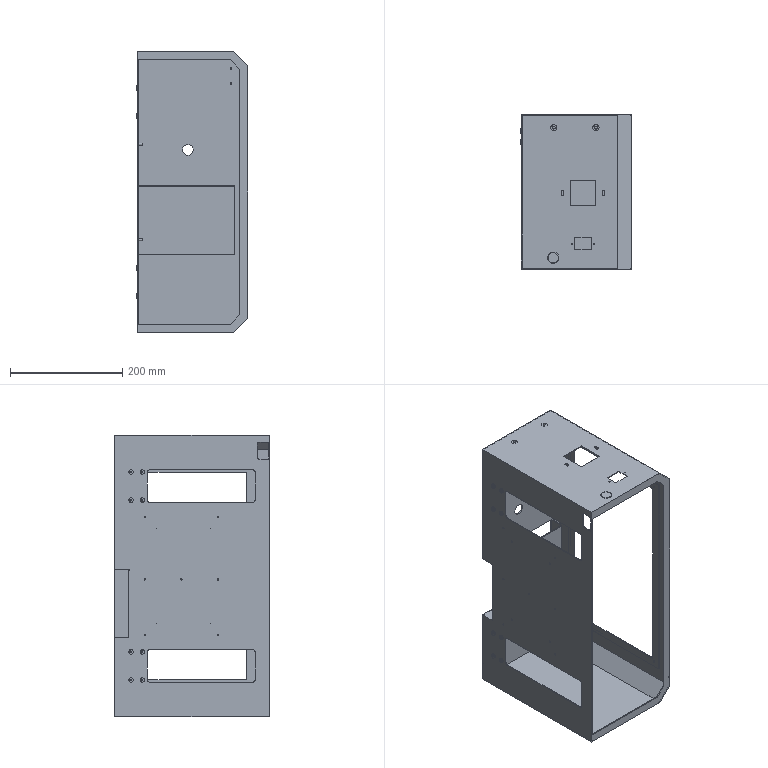Part | SolidWorks | features BaseBody 1 | 1 solid | 208 faces | box 199 x 275 x 500 mm | volume 589310 mm3 | cylinder 110 | plane 90 | cone 8 | commonest cylinder face diameters 2.5 x34 3.3 x20 7.9 x16 4.2 x8 10 x8 4.5 x4